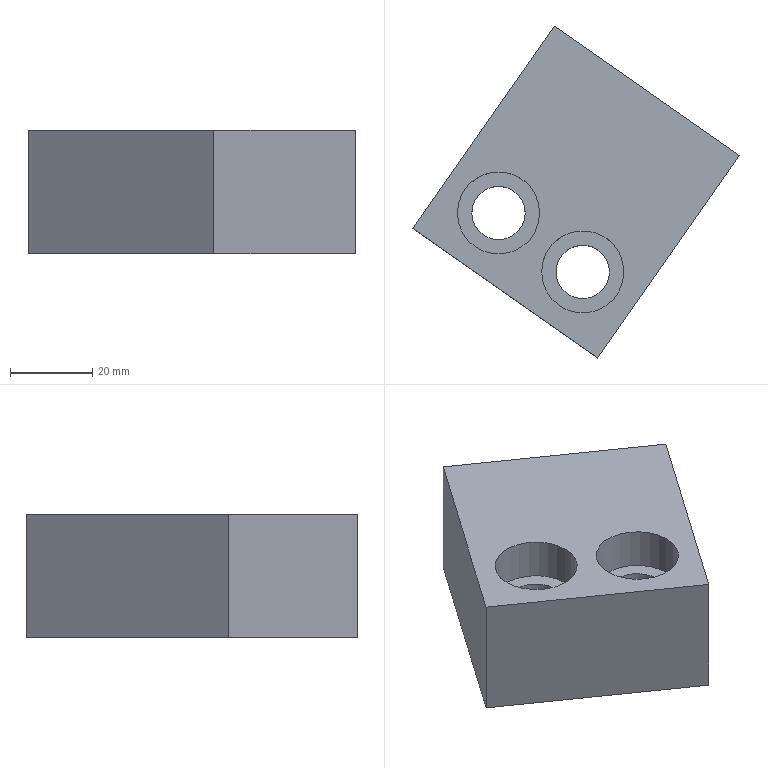Part | NX | features solid 2 | 1 solid | 12 faces | box 79.468 x 80.696 x 30 mm | volume 87408 mm3 | plane 8 | cylinder 4 | commonest cylinder face diameters 13 x2 20 x2
STEP:
#1=CARTESIAN_POINT('',(23.436,-40.826,-125.));
#2=VERTEX_POINT('',#1);
#3=CARTESIAN_POINT('',(-21.617,-9.279,-125.));
#4=VERTEX_POINT('',#3);
#5=CARTESIAN_POINT('',(19.341,-37.958,-125.));
#6=DIRECTION('',(0.8192,-0.5736,0.));
#7=VECTOR('',#6,1000.);
#8=LINE('',#5,#7);
#9=EDGE_CURVE('',#2,#4,#8,.F.);
#10=ORIENTED_EDGE('',*,*,#9,.T.);
#11=CARTESIAN_POINT('',(-21.617,-9.279,-95.));
#12=VERTEX_POINT('',#11);
#13=CARTESIAN_POINT('',(-21.617,-9.279,-100.));
#14=DIRECTION('',(0.,0.,-1.));
#15=VECTOR('',#14,1000.);
#16=LINE('',#13,#15);
#17=EDGE_CURVE('',#12,#4,#16,.T.);
#18=ORIENTED_EDGE('',*,*,#17,.F.);
#19=CARTESIAN_POINT('',(23.436,-40.826,-95.));
#20=VERTEX_POINT('',#19);
#21=CARTESIAN_POINT('',(19.341,-37.958,-95.));
#22=DIRECTION('',(0.8192,-0.5736,0.));
#23=VECTOR('',#22,1000.);
#24=LINE('',#21,#23);
#25=EDGE_CURVE('',#20,#12,#24,.F.);
#26=ORIENTED_EDGE('',*,*,#25,.F.);
#27=CARTESIAN_POINT('',(23.436,-40.826,-100.));
#28=DIRECTION('',(0.,0.,-1.));
#29=VECTOR('',#28,1000.);
#30=LINE('',#27,#29);
#31=EDGE_CURVE('',#20,#2,#30,.T.);
#32=ORIENTED_EDGE('',*,*,#31,.T.);
#33=EDGE_LOOP('',(#10,#18,#26,#32));
#34=FACE_BOUND('',#33,.T.);
#35=CARTESIAN_POINT('',(19.341,-37.958,-100.));
#36=DIRECTION('',(-0.5736,-0.8192,0.));
#37=DIRECTION('',(0.8192,-0.5736,0.));
#38=AXIS2_PLACEMENT_3D('',#35,#36,#37);
#39=PLANE('',#38);
#40=ADVANCED_FACE('',(#34),#39,.F.);
#41=CARTESIAN_POINT('',(-56.031,-58.428,-125.));
#42=VERTEX_POINT('',#41);
#43=CARTESIAN_POINT('',(245.304,371.923,-125.));
#44=DIRECTION('',(0.5736,0.8192,0.));
#45=VECTOR('',#44,1000.);
#46=LINE('',#43,#45);
#47=EDGE_CURVE('',#4,#42,#46,.F.);
#48=ORIENTED_EDGE('',*,*,#47,.T.);
#49=CARTESIAN_POINT('',(-56.031,-58.428,-95.));
#50=VERTEX_POINT('',#49);
#51=CARTESIAN_POINT('',(-56.031,-58.428,-100.));
#52=DIRECTION('',(0.,0.,-1.));
#53=VECTOR('',#52,1000.);
#54=LINE('',#51,#53);
#55=EDGE_CURVE('',#50,#42,#54,.T.);
#56=ORIENTED_EDGE('',*,*,#55,.F.);
#57=CARTESIAN_POINT('',(245.304,371.923,-95.));
#58=DIRECTION('',(0.5736,0.8192,0.));
#59=VECTOR('',#58,1000.);
#60=LINE('',#57,#59);
#61=EDGE_CURVE('',#12,#50,#60,.F.);
#62=ORIENTED_EDGE('',*,*,#61,.F.);
#63=ORIENTED_EDGE('',*,*,#17,.T.);
#64=EDGE_LOOP('',(#48,#56,#62,#63));
#65=FACE_BOUND('',#64,.T.);
#66=CARTESIAN_POINT('',(245.304,371.923,-100.));
#67=DIRECTION('',(0.8192,-0.5736,0.));
#68=DIRECTION('',(0.5736,0.8192,0.));
#69=AXIS2_PLACEMENT_3D('',#66,#67,#68);
#70=PLANE('',#69);
#71=ADVANCED_FACE('',(#65),#70,.F.);
#72=CARTESIAN_POINT('',(-10.978,-89.975,-125.));
#73=VERTEX_POINT('',#72);
#74=CARTESIAN_POINT('',(-19.17,-84.239,-125.));
#75=DIRECTION('',(0.8192,-0.5736,0.));
#76=VECTOR('',#75,1000.);
#77=LINE('',#74,#76);
#78=EDGE_CURVE('',#73,#42,#77,.F.);
#79=ORIENTED_EDGE('',*,*,#78,.F.);
#80=CARTESIAN_POINT('',(-10.978,-89.975,-95.));
#81=VERTEX_POINT('',#80);
#82=CARTESIAN_POINT('',(-10.978,-89.975,-100.));
#83=DIRECTION('',(0.,0.,-1.));
#84=VECTOR('',#83,1000.);
#85=LINE('',#82,#84);
#86=EDGE_CURVE('',#81,#73,#85,.T.);
#87=ORIENTED_EDGE('',*,*,#86,.F.);
#88=CARTESIAN_POINT('',(-19.17,-84.239,-95.));
#89=DIRECTION('',(0.8192,-0.5736,0.));
#90=VECTOR('',#89,1000.);
#91=LINE('',#88,#90);
#92=EDGE_CURVE('',#81,#50,#91,.F.);
#93=ORIENTED_EDGE('',*,*,#92,.T.);
#94=ORIENTED_EDGE('',*,*,#55,.T.);
#95=EDGE_LOOP('',(#79,#87,#93,#94));
#96=FACE_BOUND('',#95,.T.);
#97=CARTESIAN_POINT('',(-19.17,-84.239,-15.));
#98=DIRECTION('',(-0.5736,-0.8192,0.));
#99=DIRECTION('',(0.8192,-0.5736,0.));
#100=AXIS2_PLACEMENT_3D('',#97,#98,#99);
#101=PLANE('',#100);
#102=ADVANCED_FACE('',(#96),#101,.T.);
#103=CARTESIAN_POINT('',(29.172,-32.634,-125.));
#104=DIRECTION('',(0.5736,0.8192,0.));
#105=VECTOR('',#104,1000.);
#106=LINE('',#103,#105);
#107=EDGE_CURVE('',#2,#73,#106,.F.);
#108=ORIENTED_EDGE('',*,*,#107,.F.);
#109=ORIENTED_EDGE('',*,*,#31,.F.);
#110=CARTESIAN_POINT('',(29.172,-32.634,-95.));
#111=DIRECTION('',(0.5736,0.8192,0.));
#112=VECTOR('',#111,1000.);
#113=LINE('',#110,#112);
#114=EDGE_CURVE('',#20,#81,#113,.F.);
#115=ORIENTED_EDGE('',*,*,#114,.T.);
#116=ORIENTED_EDGE('',*,*,#86,.T.);
#117=EDGE_LOOP('',(#108,#109,#115,#116));
#118=FACE_BOUND('',#117,.T.);
#119=CARTESIAN_POINT('',(29.172,-32.634,-100.));
#120=DIRECTION('',(0.8192,-0.5736,0.));
#121=DIRECTION('',(0.5736,0.8192,0.));
#122=AXIS2_PLACEMENT_3D('',#119,#120,#121);
#123=PLANE('',#122);
#124=ADVANCED_FACE('',(#118),#123,.T.);
#125=CARTESIAN_POINT('',(-24.662,-69.084,-95.));
#126=VERTEX_POINT('',#125);
#127=CARTESIAN_POINT('',(-14.662,-69.084,-95.));
#128=DIRECTION('',(0.,0.,-1.));
#129=DIRECTION('',(-1.,0.,0.));
#130=AXIS2_PLACEMENT_3D('',#127,#128,#129);
#131=CIRCLE('',#130,10.);
#132=EDGE_CURVE('',#126,#126,#131,.F.);
#133=ORIENTED_EDGE('',*,*,#132,.F.);
#134=EDGE_LOOP('',(#133));
#135=FACE_BOUND('',#134,.T.);
#136=CARTESIAN_POINT('',(-45.141,-54.745,-95.));
#137=VERTEX_POINT('',#136);
#138=CARTESIAN_POINT('',(-35.141,-54.745,-95.));
#139=DIRECTION('',(0.,0.,-1.));
#140=DIRECTION('',(-1.,0.,0.));
#141=AXIS2_PLACEMENT_3D('',#138,#139,#140);
#142=CIRCLE('',#141,10.);
#143=EDGE_CURVE('',#137,#137,#142,.F.);
#144=ORIENTED_EDGE('',*,*,#143,.F.);
#145=EDGE_LOOP('',(#144));
#146=FACE_BOUND('',#145,.T.);
#147=ORIENTED_EDGE('',*,*,#25,.T.);
#148=ORIENTED_EDGE('',*,*,#61,.T.);
#149=ORIENTED_EDGE('',*,*,#92,.F.);
#150=ORIENTED_EDGE('',*,*,#114,.F.);
#151=EDGE_LOOP('',(#147,#148,#149,#150));
#152=FACE_BOUND('',#151,.T.);
#153=CARTESIAN_POINT('',(780.561,-2.868,-95.));
#154=DIRECTION('',(0.,0.,-1.));
#155=DIRECTION('',(-1.,0.,0.));
#156=AXIS2_PLACEMENT_3D('',#153,#154,#155);
#157=PLANE('',#156);
#158=ADVANCED_FACE('',(#135,#146,#152),#157,.F.);
#159=CARTESIAN_POINT('',(-21.162,-69.084,-125.));
#160=VERTEX_POINT('',#159);
#161=CARTESIAN_POINT('',(-14.662,-69.084,-125.));
#162=DIRECTION('',(0.,0.,-1.));
#163=DIRECTION('',(-1.,0.,0.));
#164=AXIS2_PLACEMENT_3D('',#161,#162,#163);
#165=CIRCLE('',#164,6.5);
#166=EDGE_CURVE('',#160,#160,#165,.F.);
#167=ORIENTED_EDGE('',*,*,#166,.T.);
#168=EDGE_LOOP('',(#167));
#169=FACE_BOUND('',#168,.T.);
#170=CARTESIAN_POINT('',(-41.641,-54.745,-125.));
#171=VERTEX_POINT('',#170);
#172=CARTESIAN_POINT('',(-35.141,-54.745,-125.));
#173=DIRECTION('',(0.,0.,-1.));
#174=DIRECTION('',(-1.,0.,0.));
#175=AXIS2_PLACEMENT_3D('',#172,#173,#174);
#176=CIRCLE('',#175,6.5);
#177=EDGE_CURVE('',#171,#171,#176,.F.);
#178=ORIENTED_EDGE('',*,*,#177,.T.);
#179=EDGE_LOOP('',(#178));
#180=FACE_BOUND('',#179,.T.);
#181=ORIENTED_EDGE('',*,*,#9,.F.);
#182=ORIENTED_EDGE('',*,*,#107,.T.);
#183=ORIENTED_EDGE('',*,*,#78,.T.);
#184=ORIENTED_EDGE('',*,*,#47,.F.);
#185=EDGE_LOOP('',(#181,#182,#183,#184));
#186=FACE_BOUND('',#185,.T.);
#187=CARTESIAN_POINT('',(780.561,-2.868,-125.));
#188=DIRECTION('',(0.,0.,-1.));
#189=DIRECTION('',(-1.,0.,0.));
#190=AXIS2_PLACEMENT_3D('',#187,#188,#189);
#191=PLANE('',#190);
#192=ADVANCED_FACE('',(#169,#180,#186),#191,.T.);
#193=CARTESIAN_POINT('',(-41.641,-54.745,-105.));
#194=VERTEX_POINT('',#193);
#195=CARTESIAN_POINT('',(-35.141,-54.745,-105.));
#196=DIRECTION('',(0.,0.,-1.));
#197=DIRECTION('',(-1.,0.,0.));
#198=AXIS2_PLACEMENT_3D('',#195,#196,#197);
#199=CIRCLE('',#198,6.5);
#200=EDGE_CURVE('',#194,#194,#199,.F.);
#201=ORIENTED_EDGE('',*,*,#200,.T.);
#202=EDGE_LOOP('',(#201));
#203=FACE_BOUND('',#202,.T.);
#204=ORIENTED_EDGE('',*,*,#177,.F.);
#205=EDGE_LOOP('',(#204));
#206=FACE_BOUND('',#205,.T.);
#207=CARTESIAN_POINT('',(-35.141,-54.745,-145.));
#208=DIRECTION('',(0.,0.,1.));
#209=DIRECTION('',(1.,0.,0.));
#210=AXIS2_PLACEMENT_3D('',#207,#208,#209);
#211=CYLINDRICAL_SURFACE('',#210,6.5);
#212=ADVANCED_FACE('',(#203,#206),#211,.F.);
#213=ORIENTED_EDGE('',*,*,#200,.F.);
#214=EDGE_LOOP('',(#213));
#215=FACE_BOUND('',#214,.T.);
#216=CARTESIAN_POINT('',(-25.141,-54.745,-105.));
#217=VERTEX_POINT('',#216);
#218=CARTESIAN_POINT('',(-35.141,-54.745,-105.));
#219=DIRECTION('',(0.,0.,1.));
#220=DIRECTION('',(1.,0.,0.));
#221=AXIS2_PLACEMENT_3D('',#218,#219,#220);
#222=CIRCLE('',#221,10.);
#223=EDGE_CURVE('',#217,#217,#222,.T.);
#224=ORIENTED_EDGE('',*,*,#223,.T.);
#225=EDGE_LOOP('',(#224));
#226=FACE_BOUND('',#225,.T.);
#227=CARTESIAN_POINT('',(-35.141,-54.745,-105.));
#228=DIRECTION('',(0.,0.,-1.));
#229=DIRECTION('',(-1.,0.,0.));
#230=AXIS2_PLACEMENT_3D('',#227,#228,#229);
#231=PLANE('',#230);
#232=ADVANCED_FACE('',(#215,#226),#231,.F.);
#233=ORIENTED_EDGE('',*,*,#143,.T.);
#234=EDGE_LOOP('',(#233));
#235=FACE_BOUND('',#234,.T.);
#236=ORIENTED_EDGE('',*,*,#223,.F.);
#237=EDGE_LOOP('',(#236));
#238=FACE_BOUND('',#237,.T.);
#239=CARTESIAN_POINT('',(-35.141,-54.745,-105.));
#240=DIRECTION('',(0.,0.,1.));
#241=DIRECTION('',(1.,0.,0.));
#242=AXIS2_PLACEMENT_3D('',#239,#240,#241);
#243=CYLINDRICAL_SURFACE('',#242,10.);
#244=ADVANCED_FACE('',(#235,#238),#243,.F.);
#245=CARTESIAN_POINT('',(-21.162,-69.084,-105.));
#246=VERTEX_POINT('',#245);
#247=CARTESIAN_POINT('',(-14.662,-69.084,-105.));
#248=DIRECTION('',(0.,0.,-1.));
#249=DIRECTION('',(-1.,0.,0.));
#250=AXIS2_PLACEMENT_3D('',#247,#248,#249);
#251=CIRCLE('',#250,6.5);
#252=EDGE_CURVE('',#246,#246,#251,.F.);
#253=ORIENTED_EDGE('',*,*,#252,.T.);
#254=EDGE_LOOP('',(#253));
#255=FACE_BOUND('',#254,.T.);
#256=ORIENTED_EDGE('',*,*,#166,.F.);
#257=EDGE_LOOP('',(#256));
#258=FACE_BOUND('',#257,.T.);
#259=CARTESIAN_POINT('',(-14.662,-69.084,-145.));
#260=DIRECTION('',(0.,0.,1.));
#261=DIRECTION('',(1.,0.,0.));
#262=AXIS2_PLACEMENT_3D('',#259,#260,#261);
#263=CYLINDRICAL_SURFACE('',#262,6.5);
#264=ADVANCED_FACE('',(#255,#258),#263,.F.);
#265=ORIENTED_EDGE('',*,*,#252,.F.);
#266=EDGE_LOOP('',(#265));
#267=FACE_BOUND('',#266,.T.);
#268=CARTESIAN_POINT('',(-4.662,-69.084,-105.));
#269=VERTEX_POINT('',#268);
#270=CARTESIAN_POINT('',(-14.662,-69.084,-105.));
#271=DIRECTION('',(0.,0.,1.));
#272=DIRECTION('',(1.,0.,0.));
#273=AXIS2_PLACEMENT_3D('',#270,#271,#272);
#274=CIRCLE('',#273,10.);
#275=EDGE_CURVE('',#269,#269,#274,.T.);
#276=ORIENTED_EDGE('',*,*,#275,.T.);
#277=EDGE_LOOP('',(#276));
#278=FACE_BOUND('',#277,.T.);
#279=CARTESIAN_POINT('',(-14.662,-69.084,-105.));
#280=DIRECTION('',(0.,0.,-1.));
#281=DIRECTION('',(-1.,0.,0.));
#282=AXIS2_PLACEMENT_3D('',#279,#280,#281);
#283=PLANE('',#282);
#284=ADVANCED_FACE('',(#267,#278),#283,.F.);
#285=ORIENTED_EDGE('',*,*,#132,.T.);
#286=EDGE_LOOP('',(#285));
#287=FACE_BOUND('',#286,.T.);
#288=ORIENTED_EDGE('',*,*,#275,.F.);
#289=EDGE_LOOP('',(#288));
#290=FACE_BOUND('',#289,.T.);
#291=CARTESIAN_POINT('',(-14.662,-69.084,-105.));
#292=DIRECTION('',(0.,0.,1.));
#293=DIRECTION('',(1.,0.,0.));
#294=AXIS2_PLACEMENT_3D('',#291,#292,#293);
#295=CYLINDRICAL_SURFACE('',#294,10.);
#296=ADVANCED_FACE('',(#287,#290),#295,.F.);
#297=CLOSED_SHELL('',(#40,#71,#102,#124,#158,#192,#212,#232,#244,#264,#284,#296));
#298=MANIFOLD_SOLID_BREP('',#297);
#299=(LENGTH_UNIT()NAMED_UNIT(*)SI_UNIT(.MILLI.,.METRE.));
#300=UNCERTAINTY_MEASURE_WITH_UNIT(LENGTH_MEASURE(0.00001),#299,'','');
#301=(NAMED_UNIT(*)PLANE_ANGLE_UNIT()SI_UNIT($,.RADIAN.));
#302=(NAMED_UNIT(*)SI_UNIT($,.STERADIAN.)SOLID_ANGLE_UNIT());
#303=(GEOMETRIC_REPRESENTATION_CONTEXT(3)GLOBAL_UNCERTAINTY_ASSIGNED_CONTEXT((#300))GLOBAL_UNIT_ASSIGNED_CONTEXT((#299,#301,#302))REPRESENTATION_CONTEXT('',''));
#304=ADVANCED_BREP_SHAPE_REPRESENTATION('',(#298),#303);